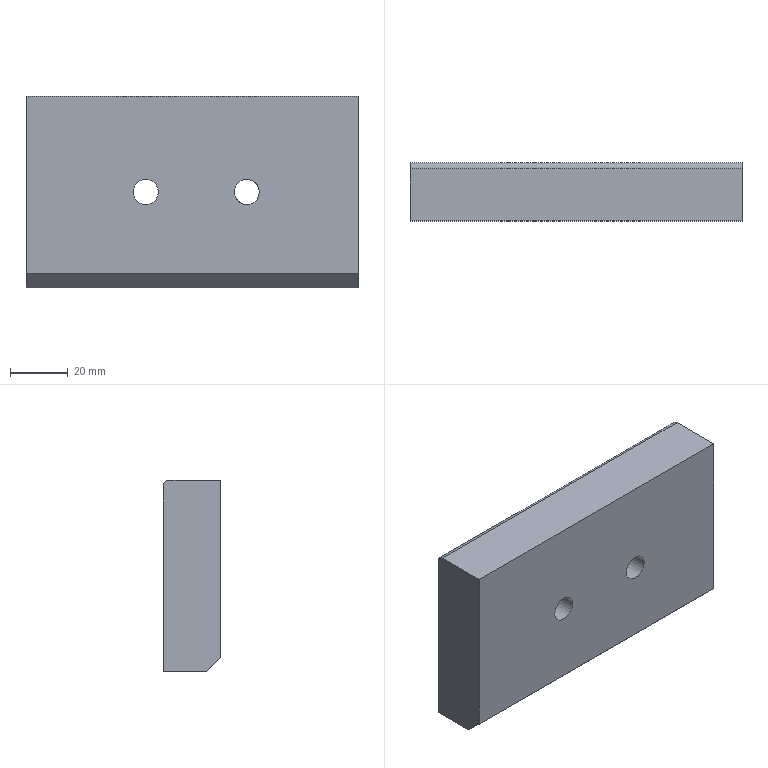Part | STEP file | 1_id1554_x_t | 1 solid | 14 faces | box 115 x 20 x 66.4 mm | volume 145757 mm3 | plane 9 | cylinder 5 | commonest cylinder face diameters 8.7 x2 15 x2 4 x1
STEP:
#1=CARTESIAN_POINT('',(0.,0.,0.));
#2=DIRECTION('',(0.,0.,1.));
#3=DIRECTION('',(1.,0.,0.));
#4=AXIS2_PLACEMENT_3D('',#1,#2,#3);
#5=CARTESIAN_POINT('',(664.7,72.624,9.122));
#6=VERTEX_POINT('',#5);
#7=CARTESIAN_POINT('',(549.7,72.624,9.122));
#8=VERTEX_POINT('',#7);
#9=CARTESIAN_POINT('',(664.7,72.624,9.122));
#10=DIRECTION('',(-1.,0.,0.));
#11=VECTOR('',#10,1.);
#12=LINE('',#9,#11);
#13=CARTESIAN_POINT('',(648.7,72.624,-105.278));
#14=DIRECTION('',(0.,1.,0.));
#15=DIRECTION('',(1.,0.,0.));
#16=AXIS2_PLACEMENT_3D('',#13,#14,#15);
#17=PLANE('',#16);
#18=CARTESIAN_POINT('',(16.,-114.4));
#19=DIRECTION('',(-1.,0.));
#20=VECTOR('',#19,1.);
#21=LINE('',#18,#20);
#22=(GEOMETRIC_REPRESENTATION_CONTEXT(2)PARAMETRIC_REPRESENTATION_CONTEXT()REPRESENTATION_CONTEXT('',''));
#23=DEFINITIONAL_REPRESENTATION('',(#21),#22);
#24=PCURVE('',#17,#23);
#25=CARTESIAN_POINT('',(648.7,70.624,9.122));
#26=DIRECTION('',(1.,0.,0.));
#27=DIRECTION('',(0.,0.,1.));
#28=AXIS2_PLACEMENT_3D('',#25,#26,#27);
#29=CYLINDRICAL_SURFACE('',#28,2.);
#30=CARTESIAN_POINT('',(4.712,16.));
#31=DIRECTION('',(0.,-1.));
#32=VECTOR('',#31,1.);
#33=LINE('',#30,#32);
#34=(GEOMETRIC_REPRESENTATION_CONTEXT(2)PARAMETRIC_REPRESENTATION_CONTEXT()REPRESENTATION_CONTEXT('',''));
#35=DEFINITIONAL_REPRESENTATION('',(#33),#34);
#36=PCURVE('',#29,#35);
#37=SURFACE_CURVE('',#12,(#24,#36),.PCURVE_S1.);
#38=EDGE_CURVE('',#6,#8,#37,.T.);
#39=ORIENTED_EDGE('',*,*,#38,.F.);
#40=CARTESIAN_POINT('',(664.7,72.624,-55.278));
#41=VERTEX_POINT('',#40);
#42=CARTESIAN_POINT('',(664.7,72.624,9.122));
#43=DIRECTION('',(0.,0.,-1.));
#44=VECTOR('',#43,1.);
#45=LINE('',#42,#44);
#46=CARTESIAN_POINT('',(16.,-114.4));
#47=DIRECTION('',(0.,1.));
#48=VECTOR('',#47,1.);
#49=LINE('',#46,#48);
#50=(GEOMETRIC_REPRESENTATION_CONTEXT(2)PARAMETRIC_REPRESENTATION_CONTEXT()REPRESENTATION_CONTEXT('',''));
#51=DEFINITIONAL_REPRESENTATION('',(#49),#50);
#52=PCURVE('',#17,#51);
#53=CARTESIAN_POINT('',(664.7,62.624,-57.278));
#54=DIRECTION('',(-1.,0.,0.));
#55=DIRECTION('',(0.,0.,-1.));
#56=AXIS2_PLACEMENT_3D('',#53,#54,#55);
#57=PLANE('',#56);
#58=CARTESIAN_POINT('',(-66.4,-10.));
#59=DIRECTION('',(1.,0.));
#60=VECTOR('',#59,1.);
#61=LINE('',#58,#60);
#62=(GEOMETRIC_REPRESENTATION_CONTEXT(2)PARAMETRIC_REPRESENTATION_CONTEXT()REPRESENTATION_CONTEXT('',''));
#63=DEFINITIONAL_REPRESENTATION('',(#61),#62);
#64=PCURVE('',#57,#63);
#65=SURFACE_CURVE('',#45,(#52,#64),.PCURVE_S1.);
#66=EDGE_CURVE('',#6,#41,#65,.T.);
#67=ORIENTED_EDGE('',*,*,#66,.T.);
#68=CARTESIAN_POINT('',(549.7,72.624,-55.278));
#69=VERTEX_POINT('',#68);
#70=CARTESIAN_POINT('',(549.7,72.624,-55.278));
#71=DIRECTION('',(1.,0.,0.));
#72=VECTOR('',#71,1.);
#73=LINE('',#70,#72);
#74=CARTESIAN_POINT('',(-99.,-50.));
#75=DIRECTION('',(1.,0.));
#76=VECTOR('',#75,1.);
#77=LINE('',#74,#76);
#78=(GEOMETRIC_REPRESENTATION_CONTEXT(2)PARAMETRIC_REPRESENTATION_CONTEXT()REPRESENTATION_CONTEXT('',''));
#79=DEFINITIONAL_REPRESENTATION('',(#77),#78);
#80=PCURVE('',#17,#79);
#81=CARTESIAN_POINT('',(648.7,72.624,-55.278));
#82=DIRECTION('',(0.,0.,1.));
#83=DIRECTION('',(1.,0.,0.));
#84=AXIS2_PLACEMENT_3D('',#81,#82,#83);
#85=PLANE('',#84);
#86=CARTESIAN_POINT('',(-99.,0.));
#87=DIRECTION('',(1.,0.));
#88=VECTOR('',#87,1.);
#89=LINE('',#86,#88);
#90=(GEOMETRIC_REPRESENTATION_CONTEXT(2)PARAMETRIC_REPRESENTATION_CONTEXT()REPRESENTATION_CONTEXT('',''));
#91=DEFINITIONAL_REPRESENTATION('',(#89),#90);
#92=PCURVE('',#85,#91);
#93=SURFACE_CURVE('',#73,(#80,#92),.PCURVE_S1.);
#94=EDGE_CURVE('',#69,#41,#93,.T.);
#95=ORIENTED_EDGE('',*,*,#94,.F.);
#96=CARTESIAN_POINT('',(549.7,72.624,9.122));
#97=DIRECTION('',(0.,0.,-1.));
#98=VECTOR('',#97,1.);
#99=LINE('',#96,#98);
#100=CARTESIAN_POINT('',(-99.,-114.4));
#101=DIRECTION('',(0.,1.));
#102=VECTOR('',#101,1.);
#103=LINE('',#100,#102);
#104=(GEOMETRIC_REPRESENTATION_CONTEXT(2)PARAMETRIC_REPRESENTATION_CONTEXT()REPRESENTATION_CONTEXT('',''));
#105=DEFINITIONAL_REPRESENTATION('',(#103),#104);
#106=PCURVE('',#17,#105);
#107=CARTESIAN_POINT('',(549.7,-37.376,-57.278));
#108=DIRECTION('',(1.,0.,0.));
#109=DIRECTION('',(0.,-1.,0.));
#110=AXIS2_PLACEMENT_3D('',#107,#108,#109);
#111=PLANE('',#110);
#112=CARTESIAN_POINT('',(-110.,-66.4));
#113=DIRECTION('',(0.,1.));
#114=VECTOR('',#113,1.);
#115=LINE('',#112,#114);
#116=(GEOMETRIC_REPRESENTATION_CONTEXT(2)PARAMETRIC_REPRESENTATION_CONTEXT()REPRESENTATION_CONTEXT('',''));
#117=DEFINITIONAL_REPRESENTATION('',(#115),#116);
#118=PCURVE('',#111,#117);
#119=SURFACE_CURVE('',#99,(#106,#118),.PCURVE_S1.);
#120=EDGE_CURVE('',#8,#69,#119,.T.);
#121=ORIENTED_EDGE('',*,*,#120,.F.);
#122=EDGE_LOOP('',(#39,#67,#95,#121));
#123=FACE_BOUND('',#122,.T.);
#124=CARTESIAN_POINT('',(618.7,72.624,-22.078));
#125=VERTEX_POINT('',#124);
#126=CARTESIAN_POINT('',(626.2,72.624,-22.078));
#127=DIRECTION('',(0.,-1.,0.));
#128=DIRECTION('',(-1.,0.,0.));
#129=AXIS2_PLACEMENT_3D('',#126,#127,#128);
#130=CIRCLE('',#129,7.5);
#131=CARTESIAN_POINT('',(-30.,-83.2));
#132=CARTESIAN_POINT('',(-30.,-70.21));
#133=CARTESIAN_POINT('',(-18.75,-76.705));
#134=CARTESIAN_POINT('',(-7.5,-83.2));
#135=CARTESIAN_POINT('',(-18.75,-89.695));
#136=CARTESIAN_POINT('',(-30.,-96.19));
#137=CARTESIAN_POINT('',(-30.,-83.2));
#138=(BOUNDED_CURVE()B_SPLINE_CURVE(2,(#131,#132,#133,#134,#135,#136,#137),.UNSPECIFIED.,.T.,.F.)B_SPLINE_CURVE_WITH_KNOTS((1,2,2,2,2,1),(-2.094,0.,2.094,4.189,6.283,8.378),.UNSPECIFIED.)CURVE()GEOMETRIC_REPRESENTATION_ITEM()RATIONAL_B_SPLINE_CURVE((1.,0.5,1.,0.5,1.,0.5,1.))REPRESENTATION_ITEM(''));
#139=(GEOMETRIC_REPRESENTATION_CONTEXT(2)PARAMETRIC_REPRESENTATION_CONTEXT()REPRESENTATION_CONTEXT('',''));
#140=DEFINITIONAL_REPRESENTATION('',(#138),#139);
#141=PCURVE('',#17,#140);
#142=CARTESIAN_POINT('',(626.2,59.624,-22.078));
#143=DIRECTION('',(0.,-1.,0.));
#144=DIRECTION('',(1.,0.,0.));
#145=AXIS2_PLACEMENT_3D('',#142,#143,#144);
#146=CYLINDRICAL_SURFACE('',#145,7.5);
#147=CARTESIAN_POINT('',(3.142,-13.));
#148=DIRECTION('',(1.,0.));
#149=VECTOR('',#148,1.);
#150=LINE('',#147,#149);
#151=(GEOMETRIC_REPRESENTATION_CONTEXT(2)PARAMETRIC_REPRESENTATION_CONTEXT()REPRESENTATION_CONTEXT('',''));
#152=DEFINITIONAL_REPRESENTATION('',(#150),#151);
#153=PCURVE('',#146,#152);
#154=SURFACE_CURVE('',#130,(#141,#153),.PCURVE_S1.);
#155=EDGE_CURVE('',#125,#125,#154,.T.);
#156=ORIENTED_EDGE('',*,*,#155,.T.);
#157=EDGE_LOOP('',(#156));
#158=FACE_BOUND('',#157,.T.);
#159=CARTESIAN_POINT('',(591.2,72.624,-29.578));
#160=VERTEX_POINT('',#159);
#161=CARTESIAN_POINT('',(591.2,72.624,-22.078));
#162=DIRECTION('',(0.,-1.,0.));
#163=DIRECTION('',(0.,0.,-1.));
#164=AXIS2_PLACEMENT_3D('',#161,#162,#163);
#165=CIRCLE('',#164,7.5);
#166=CARTESIAN_POINT('',(-57.5,-75.7));
#167=CARTESIAN_POINT('',(-44.51,-75.7));
#168=CARTESIAN_POINT('',(-51.005,-86.95));
#169=CARTESIAN_POINT('',(-57.5,-98.2));
#170=CARTESIAN_POINT('',(-63.995,-86.95));
#171=CARTESIAN_POINT('',(-70.49,-75.7));
#172=CARTESIAN_POINT('',(-57.5,-75.7));
#173=(BOUNDED_CURVE()B_SPLINE_CURVE(2,(#166,#167,#168,#169,#170,#171,#172),.UNSPECIFIED.,.T.,.F.)B_SPLINE_CURVE_WITH_KNOTS((1,2,2,2,2,1),(-2.094,0.,2.094,4.189,6.283,8.378),.UNSPECIFIED.)CURVE()GEOMETRIC_REPRESENTATION_ITEM()RATIONAL_B_SPLINE_CURVE((1.,0.5,1.,0.5,1.,0.5,1.))REPRESENTATION_ITEM(''));
#174=(GEOMETRIC_REPRESENTATION_CONTEXT(2)PARAMETRIC_REPRESENTATION_CONTEXT()REPRESENTATION_CONTEXT('',''));
#175=DEFINITIONAL_REPRESENTATION('',(#173),#174);
#176=PCURVE('',#17,#175);
#177=CARTESIAN_POINT('',(591.2,59.624,-22.078));
#178=DIRECTION('',(0.,-1.,0.));
#179=DIRECTION('',(0.,0.,1.));
#180=AXIS2_PLACEMENT_3D('',#177,#178,#179);
#181=CYLINDRICAL_SURFACE('',#180,7.5);
#182=CARTESIAN_POINT('',(3.142,-13.));
#183=DIRECTION('',(1.,0.));
#184=VECTOR('',#183,1.);
#185=LINE('',#182,#184);
#186=(GEOMETRIC_REPRESENTATION_CONTEXT(2)PARAMETRIC_REPRESENTATION_CONTEXT()REPRESENTATION_CONTEXT('',''));
#187=DEFINITIONAL_REPRESENTATION('',(#185),#186);
#188=PCURVE('',#181,#187);
#189=SURFACE_CURVE('',#165,(#176,#188),.PCURVE_S1.);
#190=EDGE_CURVE('',#160,#160,#189,.T.);
#191=ORIENTED_EDGE('',*,*,#190,.T.);
#192=EDGE_LOOP('',(#191));
#193=FACE_BOUND('',#192,.T.);
#194=ADVANCED_FACE('',(#123,#158,#193),#17,.T.);
#195=CARTESIAN_POINT('',(549.7,52.624,11.122));
#196=VERTEX_POINT('',#195);
#197=CARTESIAN_POINT('',(549.7,70.624,11.122));
#198=VERTEX_POINT('',#197);
#199=CARTESIAN_POINT('',(549.7,52.624,11.122));
#200=DIRECTION('',(0.,1.,0.));
#201=VECTOR('',#200,1.);
#202=LINE('',#199,#201);
#203=CARTESIAN_POINT('',(-90.,-68.4));
#204=DIRECTION('',(-1.,0.));
#205=VECTOR('',#204,1.);
#206=LINE('',#203,#205);
#207=(GEOMETRIC_REPRESENTATION_CONTEXT(2)PARAMETRIC_REPRESENTATION_CONTEXT()REPRESENTATION_CONTEXT('',''));
#208=DEFINITIONAL_REPRESENTATION('',(#206),#207);
#209=PCURVE('',#111,#208);
#210=CARTESIAN_POINT('',(648.7,72.624,11.122));
#211=DIRECTION('',(0.,0.,1.));
#212=DIRECTION('',(1.,0.,0.));
#213=AXIS2_PLACEMENT_3D('',#210,#211,#212);
#214=PLANE('',#213);
#215=CARTESIAN_POINT('',(-99.,-20.));
#216=DIRECTION('',(0.,1.));
#217=VECTOR('',#216,1.);
#218=LINE('',#215,#217);
#219=(GEOMETRIC_REPRESENTATION_CONTEXT(2)PARAMETRIC_REPRESENTATION_CONTEXT()REPRESENTATION_CONTEXT('',''));
#220=DEFINITIONAL_REPRESENTATION('',(#218),#219);
#221=PCURVE('',#214,#220);
#222=SURFACE_CURVE('',#202,(#209,#221),.PCURVE_S1.);
#223=EDGE_CURVE('',#196,#198,#222,.T.);
#224=ORIENTED_EDGE('',*,*,#223,.T.);
#225=CARTESIAN_POINT('',(549.7,70.624,9.122));
#226=DIRECTION('',(-1.,0.,0.));
#227=DIRECTION('',(0.,0.,1.));
#228=AXIS2_PLACEMENT_3D('',#225,#226,#227);
#229=CIRCLE('',#228,2.);
#230=CARTESIAN_POINT('',(-108.,-68.4));
#231=CARTESIAN_POINT('',(-111.464,-68.4));
#232=CARTESIAN_POINT('',(-109.732,-65.4));
#233=CARTESIAN_POINT('',(-108.,-62.4));
#234=CARTESIAN_POINT('',(-106.268,-65.4));
#235=CARTESIAN_POINT('',(-104.536,-68.4));
#236=CARTESIAN_POINT('',(-108.,-68.4));
#237=(BOUNDED_CURVE()B_SPLINE_CURVE(2,(#230,#231,#232,#233,#234,#235,#236),.UNSPECIFIED.,.T.,.F.)B_SPLINE_CURVE_WITH_KNOTS((1,2,2,2,2,1),(-2.094,0.,2.094,4.189,6.283,8.378),.UNSPECIFIED.)CURVE()GEOMETRIC_REPRESENTATION_ITEM()RATIONAL_B_SPLINE_CURVE((1.,0.5,1.,0.5,1.,0.5,1.))REPRESENTATION_ITEM(''));
#238=(GEOMETRIC_REPRESENTATION_CONTEXT(2)PARAMETRIC_REPRESENTATION_CONTEXT()REPRESENTATION_CONTEXT('',''));
#239=DEFINITIONAL_REPRESENTATION('',(#237),#238);
#240=PCURVE('',#111,#239);
#241=CARTESIAN_POINT('',(6.283,-99.));
#242=DIRECTION('',(-1.,0.));
#243=VECTOR('',#242,1.);
#244=LINE('',#241,#243);
#245=(GEOMETRIC_REPRESENTATION_CONTEXT(2)PARAMETRIC_REPRESENTATION_CONTEXT()REPRESENTATION_CONTEXT('',''));
#246=DEFINITIONAL_REPRESENTATION('',(#244),#245);
#247=PCURVE('',#29,#246);
#248=SURFACE_CURVE('',#229,(#240,#247),.PCURVE_S1.);
#249=EDGE_CURVE('',#198,#8,#248,.T.);
#250=ORIENTED_EDGE('',*,*,#249,.T.);
#251=ORIENTED_EDGE('',*,*,#120,.T.);
#252=CARTESIAN_POINT('',(549.7,57.624,-55.278));
#253=VERTEX_POINT('',#252);
#254=CARTESIAN_POINT('',(549.7,57.624,-55.278));
#255=DIRECTION('',(0.,1.,0.));
#256=VECTOR('',#255,1.);
#257=LINE('',#254,#256);
#258=CARTESIAN_POINT('',(-95.,-2.));
#259=DIRECTION('',(-1.,0.));
#260=VECTOR('',#259,1.);
#261=LINE('',#258,#260);
#262=(GEOMETRIC_REPRESENTATION_CONTEXT(2)PARAMETRIC_REPRESENTATION_CONTEXT()REPRESENTATION_CONTEXT('',''));
#263=DEFINITIONAL_REPRESENTATION('',(#261),#262);
#264=PCURVE('',#111,#263);
#265=CARTESIAN_POINT('',(-99.,-15.));
#266=DIRECTION('',(0.,1.));
#267=VECTOR('',#266,1.);
#268=LINE('',#265,#267);
#269=(GEOMETRIC_REPRESENTATION_CONTEXT(2)PARAMETRIC_REPRESENTATION_CONTEXT()REPRESENTATION_CONTEXT('',''));
#270=DEFINITIONAL_REPRESENTATION('',(#268),#269);
#271=PCURVE('',#85,#270);
#272=SURFACE_CURVE('',#257,(#264,#271),.PCURVE_S1.);
#273=EDGE_CURVE('',#253,#69,#272,.T.);
#274=ORIENTED_EDGE('',*,*,#273,.F.);
#275=CARTESIAN_POINT('',(549.7,52.624,-50.278));
#276=VERTEX_POINT('',#275);
#277=CARTESIAN_POINT('',(549.7,57.624,-55.278));
#278=DIRECTION('',(0.,-0.7071,0.7071));
#279=VECTOR('',#278,1.);
#280=LINE('',#277,#279);
#281=CARTESIAN_POINT('',(-95.,-2.));
#282=DIRECTION('',(0.7071,-0.7071));
#283=VECTOR('',#282,1.);
#284=LINE('',#281,#283);
#285=(GEOMETRIC_REPRESENTATION_CONTEXT(2)PARAMETRIC_REPRESENTATION_CONTEXT()REPRESENTATION_CONTEXT('',''));
#286=DEFINITIONAL_REPRESENTATION('',(#284),#285);
#287=PCURVE('',#111,#286);
#288=CARTESIAN_POINT('',(648.7,57.624,-55.278));
#289=DIRECTION('',(0.,-0.7071,-0.7071));
#290=DIRECTION('',(0.,0.7071,-0.7071));
#291=AXIS2_PLACEMENT_3D('',#288,#289,#290);
#292=PLANE('',#291);
#293=CARTESIAN_POINT('',(0.,-99.));
#294=DIRECTION('',(-1.,0.));
#295=VECTOR('',#294,1.);
#296=LINE('',#293,#295);
#297=(GEOMETRIC_REPRESENTATION_CONTEXT(2)PARAMETRIC_REPRESENTATION_CONTEXT()REPRESENTATION_CONTEXT('',''));
#298=DEFINITIONAL_REPRESENTATION('',(#296),#297);
#299=PCURVE('',#292,#298);
#300=SURFACE_CURVE('',#280,(#287,#299),.PCURVE_S1.);
#301=EDGE_CURVE('',#253,#276,#300,.T.);
#302=ORIENTED_EDGE('',*,*,#301,.T.);
#303=CARTESIAN_POINT('',(549.7,52.624,11.122));
#304=DIRECTION('',(0.,0.,-1.));
#305=VECTOR('',#304,1.);
#306=LINE('',#303,#305);
#307=CARTESIAN_POINT('',(-90.,-68.4));
#308=DIRECTION('',(0.,1.));
#309=VECTOR('',#308,1.);
#310=LINE('',#307,#309);
#311=(GEOMETRIC_REPRESENTATION_CONTEXT(2)PARAMETRIC_REPRESENTATION_CONTEXT()REPRESENTATION_CONTEXT('',''));
#312=DEFINITIONAL_REPRESENTATION('',(#310),#311);
#313=PCURVE('',#111,#312);
#314=CARTESIAN_POINT('',(568.7,52.624,-105.278));
#315=DIRECTION('',(0.,-1.,0.));
#316=DIRECTION('',(0.,0.,1.));
#317=AXIS2_PLACEMENT_3D('',#314,#315,#316);
#318=PLANE('',#317);
#319=CARTESIAN_POINT('',(116.4,19.));
#320=DIRECTION('',(-1.,0.));
#321=VECTOR('',#320,1.);
#322=LINE('',#319,#321);
#323=(GEOMETRIC_REPRESENTATION_CONTEXT(2)PARAMETRIC_REPRESENTATION_CONTEXT()REPRESENTATION_CONTEXT('',''));
#324=DEFINITIONAL_REPRESENTATION('',(#322),#323);
#325=PCURVE('',#318,#324);
#326=SURFACE_CURVE('',#306,(#313,#325),.PCURVE_S1.);
#327=EDGE_CURVE('',#196,#276,#326,.T.);
#328=ORIENTED_EDGE('',*,*,#327,.F.);
#329=EDGE_LOOP('',(#224,#250,#251,#274,#302,#328));
#330=FACE_BOUND('',#329,.T.);
#331=ADVANCED_FACE('',(#330),#111,.F.);
#332=CARTESIAN_POINT('',(664.7,52.624,11.122));
#333=VERTEX_POINT('',#332);
#334=CARTESIAN_POINT('',(664.7,52.624,11.122));
#335=DIRECTION('',(-1.,0.,0.));
#336=VECTOR('',#335,1.);
#337=LINE('',#334,#336);
#338=CARTESIAN_POINT('',(116.4,-96.));
#339=DIRECTION('',(0.,1.));
#340=VECTOR('',#339,1.);
#341=LINE('',#338,#340);
#342=(GEOMETRIC_REPRESENTATION_CONTEXT(2)PARAMETRIC_REPRESENTATION_CONTEXT()REPRESENTATION_CONTEXT('',''));
#343=DEFINITIONAL_REPRESENTATION('',(#341),#342);
#344=PCURVE('',#318,#343);
#345=CARTESIAN_POINT('',(16.,-20.));
#346=DIRECTION('',(-1.,0.));
#347=VECTOR('',#346,1.);
#348=LINE('',#345,#347);
#349=(GEOMETRIC_REPRESENTATION_CONTEXT(2)PARAMETRIC_REPRESENTATION_CONTEXT()REPRESENTATION_CONTEXT('',''));
#350=DEFINITIONAL_REPRESENTATION('',(#348),#349);
#351=PCURVE('',#214,#350);
#352=SURFACE_CURVE('',#337,(#344,#351),.PCURVE_S1.);
#353=EDGE_CURVE('',#333,#196,#352,.T.);
#354=ORIENTED_EDGE('',*,*,#353,.T.);
#355=ORIENTED_EDGE('',*,*,#327,.T.);
#356=CARTESIAN_POINT('',(664.7,52.624,-50.278));
#357=VERTEX_POINT('',#356);
#358=CARTESIAN_POINT('',(549.7,52.624,-50.278));
#359=DIRECTION('',(1.,0.,0.));
#360=VECTOR('',#359,1.);
#361=LINE('',#358,#360);
#362=CARTESIAN_POINT('',(55.,19.));
#363=DIRECTION('',(0.,-1.));
#364=VECTOR('',#363,1.);
#365=LINE('',#362,#364);
#366=(GEOMETRIC_REPRESENTATION_CONTEXT(2)PARAMETRIC_REPRESENTATION_CONTEXT()REPRESENTATION_CONTEXT('',''));
#367=DEFINITIONAL_REPRESENTATION('',(#365),#366);
#368=PCURVE('',#318,#367);
#369=CARTESIAN_POINT('',(-7.071,-99.));
#370=DIRECTION('',(0.,1.));
#371=VECTOR('',#370,1.);
#372=LINE('',#369,#371);
#373=(GEOMETRIC_REPRESENTATION_CONTEXT(2)PARAMETRIC_REPRESENTATION_CONTEXT()REPRESENTATION_CONTEXT('',''));
#374=DEFINITIONAL_REPRESENTATION('',(#372),#373);
#375=PCURVE('',#292,#374);
#376=SURFACE_CURVE('',#361,(#368,#375),.PCURVE_S1.);
#377=EDGE_CURVE('',#276,#357,#376,.T.);
#378=ORIENTED_EDGE('',*,*,#377,.T.);
#379=CARTESIAN_POINT('',(664.7,52.624,11.122));
#380=DIRECTION('',(0.,0.,-1.));
#381=VECTOR('',#380,1.);
#382=LINE('',#379,#381);
#383=CARTESIAN_POINT('',(116.4,-96.));
#384=DIRECTION('',(-1.,0.));
#385=VECTOR('',#384,1.);
#386=LINE('',#383,#385);
#387=(GEOMETRIC_REPRESENTATION_CONTEXT(2)PARAMETRIC_REPRESENTATION_CONTEXT()REPRESENTATION_CONTEXT('',''));
#388=DEFINITIONAL_REPRESENTATION('',(#386),#387);
#389=PCURVE('',#318,#388);
#390=CARTESIAN_POINT('',(-68.4,10.));
#391=DIRECTION('',(1.,0.));
#392=VECTOR('',#391,1.);
#393=LINE('',#390,#392);
#394=(GEOMETRIC_REPRESENTATION_CONTEXT(2)PARAMETRIC_REPRESENTATION_CONTEXT()REPRESENTATION_CONTEXT('',''));
#395=DEFINITIONAL_REPRESENTATION('',(#393),#394);
#396=PCURVE('',#57,#395);
#397=SURFACE_CURVE('',#382,(#389,#396),.PCURVE_S1.);
#398=EDGE_CURVE('',#333,#357,#397,.T.);
#399=ORIENTED_EDGE('',*,*,#398,.F.);
#400=EDGE_LOOP('',(#354,#355,#378,#399));
#401=FACE_BOUND('',#400,.T.);
#402=CARTESIAN_POINT('',(591.2,52.624,-26.428));
#403=VERTEX_POINT('',#402);
#404=CARTESIAN_POINT('',(591.2,52.624,-17.728));
#405=VERTEX_POINT('',#404);
#406=CARTESIAN_POINT('',(591.2,52.624,-22.078));
#407=DIRECTION('',(0.,1.,0.));
#408=DIRECTION('',(0.,0.,-1.));
#409=AXIS2_PLACEMENT_3D('',#406,#407,#408);
#410=CIRCLE('',#409,4.35);
#411=CARTESIAN_POINT('',(78.85,-22.5));
#412=CARTESIAN_POINT('',(78.85,-14.966));
#413=CARTESIAN_POINT('',(85.375,-18.733));
#414=CARTESIAN_POINT('',(91.9,-22.5));
#415=CARTESIAN_POINT('',(85.375,-26.267));
#416=CARTESIAN_POINT('',(78.85,-30.034));
#417=CARTESIAN_POINT('',(78.85,-22.5));
#418=(BOUNDED_CURVE()B_SPLINE_CURVE(2,(#411,#412,#413,#414,#415,#416,#417),.UNSPECIFIED.,.T.,.F.)B_SPLINE_CURVE_WITH_KNOTS((1,2,2,2,2,1),(-2.094,0.,2.094,4.189,6.283,8.378),.UNSPECIFIED.)CURVE()GEOMETRIC_REPRESENTATION_ITEM()RATIONAL_B_SPLINE_CURVE((1.,0.5,1.,0.5,1.,0.5,1.))REPRESENTATION_ITEM(''));
#419=(GEOMETRIC_REPRESENTATION_CONTEXT(2)PARAMETRIC_REPRESENTATION_CONTEXT()REPRESENTATION_CONTEXT('',''));
#420=DEFINITIONAL_REPRESENTATION('',(#418),#419);
#421=PCURVE('',#318,#420);
#422=CARTESIAN_POINT('',(591.2,52.424,-22.078));
#423=DIRECTION('',(0.,-1.,0.));
#424=DIRECTION('',(0.,0.,1.));
#425=AXIS2_PLACEMENT_3D('',#422,#423,#424);
#426=CYLINDRICAL_SURFACE('',#425,4.35);
#427=CARTESIAN_POINT('',(3.142,-0.2));
#428=DIRECTION('',(-1.,0.));
#429=VECTOR('',#428,1.);
#430=LINE('',#427,#429);
#431=(GEOMETRIC_REPRESENTATION_CONTEXT(2)PARAMETRIC_REPRESENTATION_CONTEXT()REPRESENTATION_CONTEXT('',''));
#432=DEFINITIONAL_REPRESENTATION('',(#430),#431);
#433=PCURVE('',#426,#432);
#434=SURFACE_CURVE('',#410,(#421,#433),.PCURVE_S1.);
#435=EDGE_CURVE('',#403,#405,#434,.T.);
#436=ORIENTED_EDGE('',*,*,#435,.T.);
#437=CARTESIAN_POINT('',(591.2,52.624,-22.078));
#438=DIRECTION('',(0.,1.,0.));
#439=DIRECTION('',(0.,0.,-1.));
#440=AXIS2_PLACEMENT_3D('',#437,#438,#439);
#441=CIRCLE('',#440,4.35);
#442=CARTESIAN_POINT('',(78.85,-22.5));
#443=CARTESIAN_POINT('',(78.85,-14.966));
#444=CARTESIAN_POINT('',(85.375,-18.733));
#445=CARTESIAN_POINT('',(91.9,-22.5));
#446=CARTESIAN_POINT('',(85.375,-26.267));
#447=CARTESIAN_POINT('',(78.85,-30.034));
#448=CARTESIAN_POINT('',(78.85,-22.5));
#449=(BOUNDED_CURVE()B_SPLINE_CURVE(2,(#442,#443,#444,#445,#446,#447,#448),.UNSPECIFIED.,.T.,.F.)B_SPLINE_CURVE_WITH_KNOTS((1,2,2,2,2,1),(-2.094,0.,2.094,4.189,6.283,8.378),.UNSPECIFIED.)CURVE()GEOMETRIC_REPRESENTATION_ITEM()RATIONAL_B_SPLINE_CURVE((1.,0.5,1.,0.5,1.,0.5,1.))REPRESENTATION_ITEM(''));
#450=(GEOMETRIC_REPRESENTATION_CONTEXT(2)PARAMETRIC_REPRESENTATION_CONTEXT()REPRESENTATION_CONTEXT('',''));
#451=DEFINITIONAL_REPRESENTATION('',(#449),#450);
#452=PCURVE('',#318,#451);
#453=CARTESIAN_POINT('',(9.425,-0.2));
#454=DIRECTION('',(-1.,0.));
#455=VECTOR('',#454,1.);
#456=LINE('',#453,#455);
#457=(GEOMETRIC_REPRESENTATION_CONTEXT(2)PARAMETRIC_REPRESENTATION_CONTEXT()REPRESENTATION_CONTEXT('',''));
#458=DEFINITIONAL_REPRESENTATION('',(#456),#457);
#459=PCURVE('',#426,#458);
#460=SURFACE_CURVE('',#441,(#452,#459),.PCURVE_S1.);
#461=EDGE_CURVE('',#405,#403,#460,.T.);
#462=ORIENTED_EDGE('',*,*,#461,.T.);
#463=EDGE_LOOP('',(#436,#462));
#464=FACE_BOUND('',#463,.T.);
#465=CARTESIAN_POINT('',(626.2,52.624,-26.428));
#466=VERTEX_POINT('',#465);
#467=CARTESIAN_POINT('',(626.2,52.624,-22.078));
#468=DIRECTION('',(0.,1.,0.));
#469=DIRECTION('',(0.,0.,-1.));
#470=AXIS2_PLACEMENT_3D('',#467,#468,#469);
#471=CIRCLE('',#470,4.35);
#472=CARTESIAN_POINT('',(78.85,-57.5));
#473=CARTESIAN_POINT('',(78.85,-49.966));
#474=CARTESIAN_POINT('',(85.375,-53.733));
#475=CARTESIAN_POINT('',(91.9,-57.5));
#476=CARTESIAN_POINT('',(85.375,-61.267));
#477=CARTESIAN_POINT('',(78.85,-65.034));
#478=CARTESIAN_POINT('',(78.85,-57.5));
#479=(BOUNDED_CURVE()B_SPLINE_CURVE(2,(#472,#473,#474,#475,#476,#477,#478),.UNSPECIFIED.,.T.,.F.)B_SPLINE_CURVE_WITH_KNOTS((1,2,2,2,2,1),(-2.094,0.,2.094,4.189,6.283,8.378),.UNSPECIFIED.)CURVE()GEOMETRIC_REPRESENTATION_ITEM()RATIONAL_B_SPLINE_CURVE((1.,0.5,1.,0.5,1.,0.5,1.))REPRESENTATION_ITEM(''));
#480=(GEOMETRIC_REPRESENTATION_CONTEXT(2)PARAMETRIC_REPRESENTATION_CONTEXT()REPRESENTATION_CONTEXT('',''));
#481=DEFINITIONAL_REPRESENTATION('',(#479),#480);
#482=PCURVE('',#318,#481);
#483=CARTESIAN_POINT('',(626.2,52.424,-22.078));
#484=DIRECTION('',(0.,-1.,0.));
#485=DIRECTION('',(1.,0.,0.));
#486=AXIS2_PLACEMENT_3D('',#483,#484,#485);
#487=CYLINDRICAL_SURFACE('',#486,4.35);
#488=CARTESIAN_POINT('',(10.996,-0.2));
#489=DIRECTION('',(-1.,0.));
#490=VECTOR('',#489,1.);
#491=LINE('',#488,#490);
#492=(GEOMETRIC_REPRESENTATION_CONTEXT(2)PARAMETRIC_REPRESENTATION_CONTEXT()REPRESENTATION_CONTEXT('',''));
#493=DEFINITIONAL_REPRESENTATION('',(#491),#492);
#494=PCURVE('',#487,#493);
#495=SURFACE_CURVE('',#471,(#482,#494),.PCURVE_S1.);
#496=EDGE_CURVE('',#466,#466,#495,.T.);
#497=ORIENTED_EDGE('',*,*,#496,.T.);
#498=EDGE_LOOP('',(#497));
#499=FACE_BOUND('',#498,.T.);
#500=ADVANCED_FACE('',(#401,#464,#499),#318,.T.);
#501=ORIENTED_EDGE('',*,*,#66,.F.);
#502=CARTESIAN_POINT('',(664.7,70.624,11.122));
#503=VERTEX_POINT('',#502);
#504=CARTESIAN_POINT('',(664.7,70.624,9.122));
#505=DIRECTION('',(1.,0.,0.));
#506=DIRECTION('',(0.,1.,0.));
#507=AXIS2_PLACEMENT_3D('',#504,#505,#506);
#508=CIRCLE('',#507,2.);
#509=CARTESIAN_POINT('',(-66.4,-10.));
#510=CARTESIAN_POINT('',(-69.864,-10.));
#511=CARTESIAN_POINT('',(-68.132,-7.));
#512=CARTESIAN_POINT('',(-66.4,-4.));
#513=CARTESIAN_POINT('',(-64.668,-7.));
#514=CARTESIAN_POINT('',(-62.936,-10.));
#515=CARTESIAN_POINT('',(-66.4,-10.));
#516=(BOUNDED_CURVE()B_SPLINE_CURVE(2,(#509,#510,#511,#512,#513,#514,#515),.UNSPECIFIED.,.T.,.F.)B_SPLINE_CURVE_WITH_KNOTS((1,2,2,2,2,1),(-2.094,0.,2.094,4.189,6.283,8.378),.UNSPECIFIED.)CURVE()GEOMETRIC_REPRESENTATION_ITEM()RATIONAL_B_SPLINE_CURVE((1.,0.5,1.,0.5,1.,0.5,1.))REPRESENTATION_ITEM(''));
#517=(GEOMETRIC_REPRESENTATION_CONTEXT(2)PARAMETRIC_REPRESENTATION_CONTEXT()REPRESENTATION_CONTEXT('',''));
#518=DEFINITIONAL_REPRESENTATION('',(#516),#517);
#519=PCURVE('',#57,#518);
#520=CARTESIAN_POINT('',(4.712,16.));
#521=DIRECTION('',(1.,0.));
#522=VECTOR('',#521,1.);
#523=LINE('',#520,#522);
#524=(GEOMETRIC_REPRESENTATION_CONTEXT(2)PARAMETRIC_REPRESENTATION_CONTEXT()REPRESENTATION_CONTEXT('',''));
#525=DEFINITIONAL_REPRESENTATION('',(#523),#524);
#526=PCURVE('',#29,#525);
#527=SURFACE_CURVE('',#508,(#519,#526),.PCURVE_S1.);
#528=EDGE_CURVE('',#6,#503,#527,.T.);
#529=ORIENTED_EDGE('',*,*,#528,.T.);
#530=CARTESIAN_POINT('',(664.7,70.624,11.122));
#531=DIRECTION('',(0.,-1.,0.));
#532=VECTOR('',#531,1.);
#533=LINE('',#530,#532);
#534=CARTESIAN_POINT('',(-68.4,-8.));
#535=DIRECTION('',(0.,1.));
#536=VECTOR('',#535,1.);
#537=LINE('',#534,#536);
#538=(GEOMETRIC_REPRESENTATION_CONTEXT(2)PARAMETRIC_REPRESENTATION_CONTEXT()REPRESENTATION_CONTEXT('',''));
#539=DEFINITIONAL_REPRESENTATION('',(#537),#538);
#540=PCURVE('',#57,#539);
#541=CARTESIAN_POINT('',(16.,-2.));
#542=DIRECTION('',(0.,-1.));
#543=VECTOR('',#542,1.);
#544=LINE('',#541,#543);
#545=(GEOMETRIC_REPRESENTATION_CONTEXT(2)PARAMETRIC_REPRESENTATION_CONTEXT()REPRESENTATION_CONTEXT('',''));
#546=DEFINITIONAL_REPRESENTATION('',(#544),#545);
#547=PCURVE('',#214,#546);
#548=SURFACE_CURVE('',#533,(#540,#547),.PCURVE_S1.);
#549=EDGE_CURVE('',#503,#333,#548,.T.);
#550=ORIENTED_EDGE('',*,*,#549,.T.);
#551=ORIENTED_EDGE('',*,*,#398,.T.);
#552=CARTESIAN_POINT('',(664.7,57.624,-55.278));
#553=VERTEX_POINT('',#552);
#554=CARTESIAN_POINT('',(664.7,52.624,-50.278));
#555=DIRECTION('',(0.,0.7071,-0.7071));
#556=VECTOR('',#555,1.);
#557=LINE('',#554,#556);
#558=CARTESIAN_POINT('',(-7.,10.));
#559=DIRECTION('',(0.7071,-0.7071));
#560=VECTOR('',#559,1.);
#561=LINE('',#558,#560);
#562=(GEOMETRIC_REPRESENTATION_CONTEXT(2)PARAMETRIC_REPRESENTATION_CONTEXT()REPRESENTATION_CONTEXT('',''));
#563=DEFINITIONAL_REPRESENTATION('',(#561),#562);
#564=PCURVE('',#57,#563);
#565=CARTESIAN_POINT('',(-7.071,16.));
#566=DIRECTION('',(1.,0.));
#567=VECTOR('',#566,1.);
#568=LINE('',#565,#567);
#569=(GEOMETRIC_REPRESENTATION_CONTEXT(2)PARAMETRIC_REPRESENTATION_CONTEXT()REPRESENTATION_CONTEXT('',''));
#570=DEFINITIONAL_REPRESENTATION('',(#568),#569);
#571=PCURVE('',#292,#570);
#572=SURFACE_CURVE('',#557,(#564,#571),.PCURVE_S1.);
#573=EDGE_CURVE('',#357,#553,#572,.T.);
#574=ORIENTED_EDGE('',*,*,#573,.T.);
#575=CARTESIAN_POINT('',(664.7,72.624,-55.278));
#576=DIRECTION('',(0.,-1.,0.));
#577=VECTOR('',#576,1.);
#578=LINE('',#575,#577);
#579=CARTESIAN_POINT('',(-2.,-10.));
#580=DIRECTION('',(0.,1.));
#581=VECTOR('',#580,1.);
#582=LINE('',#579,#581);
#583=(GEOMETRIC_REPRESENTATION_CONTEXT(2)PARAMETRIC_REPRESENTATION_CONTEXT()REPRESENTATION_CONTEXT('',''));
#584=DEFINITIONAL_REPRESENTATION('',(#582),#583);
#585=PCURVE('',#57,#584);
#586=CARTESIAN_POINT('',(16.,0.));
#587=DIRECTION('',(0.,-1.));
#588=VECTOR('',#587,1.);
#589=LINE('',#586,#588);
#590=(GEOMETRIC_REPRESENTATION_CONTEXT(2)PARAMETRIC_REPRESENTATION_CONTEXT()REPRESENTATION_CONTEXT('',''));
#591=DEFINITIONAL_REPRESENTATION('',(#589),#590);
#592=PCURVE('',#85,#591);
#593=SURFACE_CURVE('',#578,(#585,#592),.PCURVE_S1.);
#594=EDGE_CURVE('',#41,#553,#593,.T.);
#595=ORIENTED_EDGE('',*,*,#594,.F.);
#596=EDGE_LOOP('',(#501,#529,#550,#551,#574,#595));
#597=FACE_BOUND('',#596,.T.);
#598=ADVANCED_FACE('',(#597),#57,.F.);
#599=ORIENTED_EDGE('',*,*,#94,.T.);
#600=ORIENTED_EDGE('',*,*,#594,.T.);
#601=CARTESIAN_POINT('',(664.7,57.624,-55.278));
#602=DIRECTION('',(-1.,0.,0.));
#603=VECTOR('',#602,1.);
#604=LINE('',#601,#603);
#605=CARTESIAN_POINT('',(16.,-15.));
#606=DIRECTION('',(-1.,0.));
#607=VECTOR('',#606,1.);
#608=LINE('',#605,#607);
#609=(GEOMETRIC_REPRESENTATION_CONTEXT(2)PARAMETRIC_REPRESENTATION_CONTEXT()REPRESENTATION_CONTEXT('',''));
#610=DEFINITIONAL_REPRESENTATION('',(#608),#609);
#611=PCURVE('',#85,#610);
#612=CARTESIAN_POINT('',(0.,16.));
#613=DIRECTION('',(0.,-1.));
#614=VECTOR('',#613,1.);
#615=LINE('',#612,#614);
#616=(GEOMETRIC_REPRESENTATION_CONTEXT(2)PARAMETRIC_REPRESENTATION_CONTEXT()REPRESENTATION_CONTEXT('',''));
#617=DEFINITIONAL_REPRESENTATION('',(#615),#616);
#618=PCURVE('',#292,#617);
#619=SURFACE_CURVE('',#604,(#611,#618),.PCURVE_S1.);
#620=EDGE_CURVE('',#553,#253,#619,.T.);
#621=ORIENTED_EDGE('',*,*,#620,.T.);
#622=ORIENTED_EDGE('',*,*,#273,.T.);
#623=EDGE_LOOP('',(#599,#600,#621,#622));
#624=FACE_BOUND('',#623,.T.);
#625=ADVANCED_FACE('',(#624),#85,.F.);
#626=ORIENTED_EDGE('',*,*,#620,.F.);
#627=ORIENTED_EDGE('',*,*,#573,.F.);
#628=ORIENTED_EDGE('',*,*,#377,.F.);
#629=ORIENTED_EDGE('',*,*,#301,.F.);
#630=EDGE_LOOP('',(#626,#627,#628,#629));
#631=FACE_BOUND('',#630,.T.);
#632=ADVANCED_FACE('',(#631),#292,.T.);
#633=CARTESIAN_POINT('',(549.7,70.624,11.122));
#634=DIRECTION('',(1.,0.,0.));
#635=VECTOR('',#634,1.);
#636=LINE('',#633,#635);
#637=CARTESIAN_POINT('',(-99.,-2.));
#638=DIRECTION('',(1.,0.));
#639=VECTOR('',#638,1.);
#640=LINE('',#637,#639);
#641=(GEOMETRIC_REPRESENTATION_CONTEXT(2)PARAMETRIC_REPRESENTATION_CONTEXT()REPRESENTATION_CONTEXT('',''));
#642=DEFINITIONAL_REPRESENTATION('',(#640),#641);
#643=PCURVE('',#214,#642);
#644=CARTESIAN_POINT('',(6.283,-99.));
#645=DIRECTION('',(0.,1.));
#646=VECTOR('',#645,1.);
#647=LINE('',#644,#646);
#648=(GEOMETRIC_REPRESENTATION_CONTEXT(2)PARAMETRIC_REPRESENTATION_CONTEXT()REPRESENTATION_CONTEXT('',''));
#649=DEFINITIONAL_REPRESENTATION('',(#647),#648);
#650=PCURVE('',#29,#649);
#651=SURFACE_CURVE('',#636,(#643,#650),.PCURVE_S1.);
#652=EDGE_CURVE('',#198,#503,#651,.T.);
#653=ORIENTED_EDGE('',*,*,#652,.F.);
#654=ORIENTED_EDGE('',*,*,#223,.F.);
#655=ORIENTED_EDGE('',*,*,#353,.F.);
#656=ORIENTED_EDGE('',*,*,#549,.F.);
#657=EDGE_LOOP('',(#653,#654,#655,#656));
#658=FACE_BOUND('',#657,.T.);
#659=ADVANCED_FACE('',(#658),#214,.T.);
#660=ORIENTED_EDGE('',*,*,#38,.T.);
#661=ORIENTED_EDGE('',*,*,#249,.F.);
#662=ORIENTED_EDGE('',*,*,#652,.T.);
#663=ORIENTED_EDGE('',*,*,#528,.F.);
#664=EDGE_LOOP('',(#660,#661,#662,#663));
#665=FACE_BOUND('',#664,.T.);
#666=ADVANCED_FACE('',(#665),#29,.T.);
#667=ORIENTED_EDGE('',*,*,#435,.T.);
#668=CARTESIAN_POINT('',(591.2,59.624,-17.728));
#669=VERTEX_POINT('',#668);
#670=CARTESIAN_POINT('',(591.2,59.624,-17.728));
#671=CARTESIAN_POINT('',(591.2,52.624,-17.728));
#672=B_SPLINE_CURVE_WITH_KNOTS('',1,(#670,#671),.UNSPECIFIED.,.F.,.F.,(2,2),(-7.2,-0.2),.PIECEWISE_BEZIER_KNOTS.);
#673=CARTESIAN_POINT('',(0.,0.));
#674=DIRECTION('',(0.,1.));
#675=VECTOR('',#674,1.);
#676=LINE('',#673,#675);
#677=(GEOMETRIC_REPRESENTATION_CONTEXT(2)PARAMETRIC_REPRESENTATION_CONTEXT()REPRESENTATION_CONTEXT('',''));
#678=DEFINITIONAL_REPRESENTATION('',(#676),#677);
#679=PCURVE('',#426,#678);
#680=CARTESIAN_POINT('',(6.283,0.));
#681=DIRECTION('',(0.,1.));
#682=VECTOR('',#681,1.);
#683=LINE('',#680,#682);
#684=(GEOMETRIC_REPRESENTATION_CONTEXT(2)PARAMETRIC_REPRESENTATION_CONTEXT()REPRESENTATION_CONTEXT('',''));
#685=DEFINITIONAL_REPRESENTATION('',(#683),#684);
#686=PCURVE('',#426,#685);
#687=SEAM_CURVE('',#672,(#679,#686),.PCURVE_S1.);
#688=EDGE_CURVE('',#669,#405,#687,.T.);
#689=ORIENTED_EDGE('',*,*,#688,.F.);
#690=CARTESIAN_POINT('',(591.2,59.624,-22.078));
#691=DIRECTION('',(0.,-1.,0.));
#692=DIRECTION('',(0.,0.,1.));
#693=AXIS2_PLACEMENT_3D('',#690,#691,#692);
#694=CIRCLE('',#693,4.35);
#695=CARTESIAN_POINT('',(0.,-7.2));
#696=DIRECTION('',(1.,0.));
#697=VECTOR('',#696,1.);
#698=LINE('',#695,#697);
#699=(GEOMETRIC_REPRESENTATION_CONTEXT(2)PARAMETRIC_REPRESENTATION_CONTEXT()REPRESENTATION_CONTEXT('',''));
#700=DEFINITIONAL_REPRESENTATION('',(#698),#699);
#701=PCURVE('',#426,#700);
#702=CARTESIAN_POINT('',(591.2,59.624,-22.078));
#703=DIRECTION('',(0.,-1.,0.));
#704=DIRECTION('',(0.,0.,1.));
#705=AXIS2_PLACEMENT_3D('',#702,#703,#704);
#706=PLANE('',#705);
#707=CARTESIAN_POINT('',(0.,0.));
#708=DIRECTION('',(1.,0.));
#709=AXIS2_PLACEMENT_2D('',#707,#708);
#710=CIRCLE('',#709,4.35);
#711=(GEOMETRIC_REPRESENTATION_CONTEXT(2)PARAMETRIC_REPRESENTATION_CONTEXT()REPRESENTATION_CONTEXT('',''));
#712=DEFINITIONAL_REPRESENTATION('',(#710),#711);
#713=PCURVE('',#706,#712);
#714=SURFACE_CURVE('',#694,(#701,#713),.PCURVE_S1.);
#715=EDGE_CURVE('',#669,#669,#714,.T.);
#716=ORIENTED_EDGE('',*,*,#715,.T.);
#717=ORIENTED_EDGE('',*,*,#688,.T.);
#718=ORIENTED_EDGE('',*,*,#461,.T.);
#719=EDGE_LOOP('',(#667,#689,#716,#717,#718));
#720=FACE_BOUND('',#719,.F.);
#721=ADVANCED_FACE('',(#720),#426,.F.);
#722=CARTESIAN_POINT('',(591.2,59.624,-29.578));
#723=VERTEX_POINT('',#722);
#724=CARTESIAN_POINT('',(591.2,59.624,-22.078));
#725=DIRECTION('',(0.,1.,0.));
#726=DIRECTION('',(0.,0.,-1.));
#727=AXIS2_PLACEMENT_3D('',#724,#725,#726);
#728=CIRCLE('',#727,7.5);
#729=CARTESIAN_POINT('',(-7.5,0.));
#730=CARTESIAN_POINT('',(-7.5,12.99));
#731=CARTESIAN_POINT('',(3.75,6.495));
#732=CARTESIAN_POINT('',(15.,0.));
#733=CARTESIAN_POINT('',(3.75,-6.495));
#734=CARTESIAN_POINT('',(-7.5,-12.99));
#735=CARTESIAN_POINT('',(-7.5,0.));
#736=(BOUNDED_CURVE()B_SPLINE_CURVE(2,(#729,#730,#731,#732,#733,#734,#735),.UNSPECIFIED.,.T.,.F.)B_SPLINE_CURVE_WITH_KNOTS((1,2,2,2,2,1),(-2.094,0.,2.094,4.189,6.283,8.378),.UNSPECIFIED.)CURVE()GEOMETRIC_REPRESENTATION_ITEM()RATIONAL_B_SPLINE_CURVE((1.,0.5,1.,0.5,1.,0.5,1.))REPRESENTATION_ITEM(''));
#737=(GEOMETRIC_REPRESENTATION_CONTEXT(2)PARAMETRIC_REPRESENTATION_CONTEXT()REPRESENTATION_CONTEXT('',''));
#738=DEFINITIONAL_REPRESENTATION('',(#736),#737);
#739=PCURVE('',#706,#738);
#740=CARTESIAN_POINT('',(9.425,0.));
#741=DIRECTION('',(-1.,0.));
#742=VECTOR('',#741,1.);
#743=LINE('',#740,#742);
#744=(GEOMETRIC_REPRESENTATION_CONTEXT(2)PARAMETRIC_REPRESENTATION_CONTEXT()REPRESENTATION_CONTEXT('',''));
#745=DEFINITIONAL_REPRESENTATION('',(#743),#744);
#746=PCURVE('',#181,#745);
#747=SURFACE_CURVE('',#728,(#739,#746),.PCURVE_S1.);
#748=EDGE_CURVE('',#723,#723,#747,.T.);
#749=ORIENTED_EDGE('',*,*,#748,.T.);
#750=EDGE_LOOP('',(#749));
#751=FACE_BOUND('',#750,.T.);
#752=ORIENTED_EDGE('',*,*,#715,.T.);
#753=EDGE_LOOP('',(#752));
#754=FACE_BOUND('',#753,.T.);
#755=ADVANCED_FACE('',(#751,#754),#706,.F.);
#756=ORIENTED_EDGE('',*,*,#748,.T.);
#757=CARTESIAN_POINT('',(591.2,72.624,-29.578));
#758=CARTESIAN_POINT('',(591.2,59.624,-29.578));
#759=B_SPLINE_CURVE_WITH_KNOTS('',1,(#757,#758),.UNSPECIFIED.,.F.,.F.,(2,2),(-13.,0.),.PIECEWISE_BEZIER_KNOTS.);
#760=CARTESIAN_POINT('',(3.142,0.));
#761=DIRECTION('',(0.,1.));
#762=VECTOR('',#761,1.);
#763=LINE('',#760,#762);
#764=(GEOMETRIC_REPRESENTATION_CONTEXT(2)PARAMETRIC_REPRESENTATION_CONTEXT()REPRESENTATION_CONTEXT('',''));
#765=DEFINITIONAL_REPRESENTATION('',(#763),#764);
#766=PCURVE('',#181,#765);
#767=CARTESIAN_POINT('',(9.425,0.));
#768=DIRECTION('',(0.,1.));
#769=VECTOR('',#768,1.);
#770=LINE('',#767,#769);
#771=(GEOMETRIC_REPRESENTATION_CONTEXT(2)PARAMETRIC_REPRESENTATION_CONTEXT()REPRESENTATION_CONTEXT('',''));
#772=DEFINITIONAL_REPRESENTATION('',(#770),#771);
#773=PCURVE('',#181,#772);
#774=SEAM_CURVE('',#759,(#766,#773),.PCURVE_S1.);
#775=EDGE_CURVE('',#160,#723,#774,.T.);
#776=ORIENTED_EDGE('',*,*,#775,.F.);
#777=ORIENTED_EDGE('',*,*,#190,.T.);
#778=ORIENTED_EDGE('',*,*,#775,.T.);
#779=EDGE_LOOP('',(#756,#776,#777,#778));
#780=FACE_BOUND('',#779,.F.);
#781=ADVANCED_FACE('',(#780),#181,.F.);
#782=ORIENTED_EDGE('',*,*,#496,.T.);
#783=CARTESIAN_POINT('',(626.2,59.624,-26.428));
#784=VERTEX_POINT('',#783);
#785=CARTESIAN_POINT('',(626.2,59.624,-26.428));
#786=CARTESIAN_POINT('',(626.2,52.624,-26.428));
#787=B_SPLINE_CURVE_WITH_KNOTS('',1,(#785,#786),.UNSPECIFIED.,.F.,.F.,(2,2),(-7.2,-0.2),.PIECEWISE_BEZIER_KNOTS.);
#788=CARTESIAN_POINT('',(4.712,0.));
#789=DIRECTION('',(0.,1.));
#790=VECTOR('',#789,1.);
#791=LINE('',#788,#790);
#792=(GEOMETRIC_REPRESENTATION_CONTEXT(2)PARAMETRIC_REPRESENTATION_CONTEXT()REPRESENTATION_CONTEXT('',''));
#793=DEFINITIONAL_REPRESENTATION('',(#791),#792);
#794=PCURVE('',#487,#793);
#795=CARTESIAN_POINT('',(10.996,0.));
#796=DIRECTION('',(0.,1.));
#797=VECTOR('',#796,1.);
#798=LINE('',#795,#797);
#799=(GEOMETRIC_REPRESENTATION_CONTEXT(2)PARAMETRIC_REPRESENTATION_CONTEXT()REPRESENTATION_CONTEXT('',''));
#800=DEFINITIONAL_REPRESENTATION('',(#798),#799);
#801=PCURVE('',#487,#800);
#802=SEAM_CURVE('',#787,(#794,#801),.PCURVE_S1.);
#803=EDGE_CURVE('',#784,#466,#802,.T.);
#804=ORIENTED_EDGE('',*,*,#803,.F.);
#805=CARTESIAN_POINT('',(621.85,59.624,-22.078));
#806=VERTEX_POINT('',#805);
#807=CARTESIAN_POINT('',(626.2,59.624,-22.078));
#808=DIRECTION('',(0.,-1.,0.));
#809=DIRECTION('',(-1.,0.,0.));
#810=AXIS2_PLACEMENT_3D('',#807,#808,#809);
#811=CIRCLE('',#810,4.35);
#812=CARTESIAN_POINT('',(3.142,-7.2));
#813=DIRECTION('',(1.,0.));
#814=VECTOR('',#813,1.);
#815=LINE('',#812,#814);
#816=(GEOMETRIC_REPRESENTATION_CONTEXT(2)PARAMETRIC_REPRESENTATION_CONTEXT()REPRESENTATION_CONTEXT('',''));
#817=DEFINITIONAL_REPRESENTATION('',(#815),#816);
#818=PCURVE('',#487,#817);
#819=CARTESIAN_POINT('',(626.2,59.624,-22.078));
#820=DIRECTION('',(0.,-1.,0.));
#821=DIRECTION('',(0.,0.,1.));
#822=AXIS2_PLACEMENT_3D('',#819,#820,#821);
#823=PLANE('',#822);
#824=CARTESIAN_POINT('',(0.,0.));
#825=DIRECTION('',(0.,1.));
#826=AXIS2_PLACEMENT_2D('',#824,#825);
#827=CIRCLE('',#826,4.35);
#828=(GEOMETRIC_REPRESENTATION_CONTEXT(2)PARAMETRIC_REPRESENTATION_CONTEXT()REPRESENTATION_CONTEXT('',''));
#829=DEFINITIONAL_REPRESENTATION('',(#827),#828);
#830=PCURVE('',#823,#829);
#831=SURFACE_CURVE('',#811,(#818,#830),.PCURVE_S1.);
#832=EDGE_CURVE('',#784,#806,#831,.T.);
#833=ORIENTED_EDGE('',*,*,#832,.T.);
#834=CARTESIAN_POINT('',(626.2,59.624,-22.078));
#835=DIRECTION('',(0.,-1.,0.));
#836=DIRECTION('',(-1.,0.,0.));
#837=AXIS2_PLACEMENT_3D('',#834,#835,#836);
#838=CIRCLE('',#837,4.35);
#839=CARTESIAN_POINT('',(9.425,-7.2));
#840=DIRECTION('',(1.,0.));
#841=VECTOR('',#840,1.);
#842=LINE('',#839,#841);
#843=(GEOMETRIC_REPRESENTATION_CONTEXT(2)PARAMETRIC_REPRESENTATION_CONTEXT()REPRESENTATION_CONTEXT('',''));
#844=DEFINITIONAL_REPRESENTATION('',(#842),#843);
#845=PCURVE('',#487,#844);
#846=CARTESIAN_POINT('',(0.,0.));
#847=DIRECTION('',(0.,1.));
#848=AXIS2_PLACEMENT_2D('',#846,#847);
#849=CIRCLE('',#848,4.35);
#850=(GEOMETRIC_REPRESENTATION_CONTEXT(2)PARAMETRIC_REPRESENTATION_CONTEXT()REPRESENTATION_CONTEXT('',''));
#851=DEFINITIONAL_REPRESENTATION('',(#849),#850);
#852=PCURVE('',#823,#851);
#853=SURFACE_CURVE('',#838,(#845,#852),.PCURVE_S1.);
#854=EDGE_CURVE('',#806,#784,#853,.T.);
#855=ORIENTED_EDGE('',*,*,#854,.T.);
#856=ORIENTED_EDGE('',*,*,#803,.T.);
#857=EDGE_LOOP('',(#782,#804,#833,#855,#856));
#858=FACE_BOUND('',#857,.F.);
#859=ADVANCED_FACE('',(#858),#487,.F.);
#860=CARTESIAN_POINT('',(618.7,59.624,-22.078));
#861=VERTEX_POINT('',#860);
#862=CARTESIAN_POINT('',(626.2,59.624,-22.078));
#863=DIRECTION('',(0.,1.,0.));
#864=DIRECTION('',(-1.,0.,0.));
#865=AXIS2_PLACEMENT_3D('',#862,#863,#864);
#866=CIRCLE('',#865,7.5);
#867=CARTESIAN_POINT('',(0.,7.5));
#868=CARTESIAN_POINT('',(12.99,7.5));
#869=CARTESIAN_POINT('',(6.495,-3.75));
#870=CARTESIAN_POINT('',(0.,-15.));
#871=CARTESIAN_POINT('',(-6.495,-3.75));
#872=CARTESIAN_POINT('',(-12.99,7.5));
#873=CARTESIAN_POINT('',(0.,7.5));
#874=(BOUNDED_CURVE()B_SPLINE_CURVE(2,(#867,#868,#869,#870,#871,#872,#873),.UNSPECIFIED.,.T.,.F.)B_SPLINE_CURVE_WITH_KNOTS((1,2,2,2,2,1),(-2.094,0.,2.094,4.189,6.283,8.378),.UNSPECIFIED.)CURVE()GEOMETRIC_REPRESENTATION_ITEM()RATIONAL_B_SPLINE_CURVE((1.,0.5,1.,0.5,1.,0.5,1.))REPRESENTATION_ITEM(''));
#875=(GEOMETRIC_REPRESENTATION_CONTEXT(2)PARAMETRIC_REPRESENTATION_CONTEXT()REPRESENTATION_CONTEXT('',''));
#876=DEFINITIONAL_REPRESENTATION('',(#874),#875);
#877=PCURVE('',#823,#876);
#878=CARTESIAN_POINT('',(9.425,0.));
#879=DIRECTION('',(-1.,0.));
#880=VECTOR('',#879,1.);
#881=LINE('',#878,#880);
#882=(GEOMETRIC_REPRESENTATION_CONTEXT(2)PARAMETRIC_REPRESENTATION_CONTEXT()REPRESENTATION_CONTEXT('',''));
#883=DEFINITIONAL_REPRESENTATION('',(#881),#882);
#884=PCURVE('',#146,#883);
#885=SURFACE_CURVE('',#866,(#877,#884),.PCURVE_S1.);
#886=EDGE_CURVE('',#861,#861,#885,.T.);
#887=ORIENTED_EDGE('',*,*,#886,.T.);
#888=EDGE_LOOP('',(#887));
#889=FACE_BOUND('',#888,.T.);
#890=ORIENTED_EDGE('',*,*,#854,.T.);
#891=ORIENTED_EDGE('',*,*,#832,.T.);
#892=EDGE_LOOP('',(#890,#891));
#893=FACE_BOUND('',#892,.T.);
#894=ADVANCED_FACE('',(#889,#893),#823,.F.);
#895=ORIENTED_EDGE('',*,*,#886,.T.);
#896=CARTESIAN_POINT('',(618.7,72.624,-22.078));
#897=CARTESIAN_POINT('',(618.7,59.624,-22.078));
#898=B_SPLINE_CURVE_WITH_KNOTS('',1,(#896,#897),.UNSPECIFIED.,.F.,.F.,(2,2),(-13.,0.),.PIECEWISE_BEZIER_KNOTS.);
#899=CARTESIAN_POINT('',(3.142,0.));
#900=DIRECTION('',(0.,1.));
#901=VECTOR('',#900,1.);
#902=LINE('',#899,#901);
#903=(GEOMETRIC_REPRESENTATION_CONTEXT(2)PARAMETRIC_REPRESENTATION_CONTEXT()REPRESENTATION_CONTEXT('',''));
#904=DEFINITIONAL_REPRESENTATION('',(#902),#903);
#905=PCURVE('',#146,#904);
#906=CARTESIAN_POINT('',(9.425,0.));
#907=DIRECTION('',(0.,1.));
#908=VECTOR('',#907,1.);
#909=LINE('',#906,#908);
#910=(GEOMETRIC_REPRESENTATION_CONTEXT(2)PARAMETRIC_REPRESENTATION_CONTEXT()REPRESENTATION_CONTEXT('',''));
#911=DEFINITIONAL_REPRESENTATION('',(#909),#910);
#912=PCURVE('',#146,#911);
#913=SEAM_CURVE('',#898,(#905,#912),.PCURVE_S1.);
#914=EDGE_CURVE('',#125,#861,#913,.T.);
#915=ORIENTED_EDGE('',*,*,#914,.F.);
#916=ORIENTED_EDGE('',*,*,#155,.T.);
#917=ORIENTED_EDGE('',*,*,#914,.T.);
#918=EDGE_LOOP('',(#895,#915,#916,#917));
#919=FACE_BOUND('',#918,.F.);
#920=ADVANCED_FACE('',(#919),#146,.F.);
#921=CLOSED_SHELL('',(#194,#331,#500,#598,#625,#632,#659,#666,#721,#755,#781,#859,#894,#920));
#922=MANIFOLD_SOLID_BREP('',#921);
#923=(LENGTH_UNIT()NAMED_UNIT(*)SI_UNIT(.MILLI.,.METRE.));
#924=UNCERTAINTY_MEASURE_WITH_UNIT(LENGTH_MEASURE(0.000002),#923,'','');
#925=(NAMED_UNIT(*)PLANE_ANGLE_UNIT()SI_UNIT($,.RADIAN.));
#926=(NAMED_UNIT(*)SI_UNIT($,.STERADIAN.)SOLID_ANGLE_UNIT());
#927=(GEOMETRIC_REPRESENTATION_CONTEXT(3)GLOBAL_UNCERTAINTY_ASSIGNED_CONTEXT((#924))GLOBAL_UNIT_ASSIGNED_CONTEXT((#923,#925,#926))REPRESENTATION_CONTEXT('',''));
#928=ADVANCED_BREP_SHAPE_REPRESENTATION('',(#4,#922),#927);